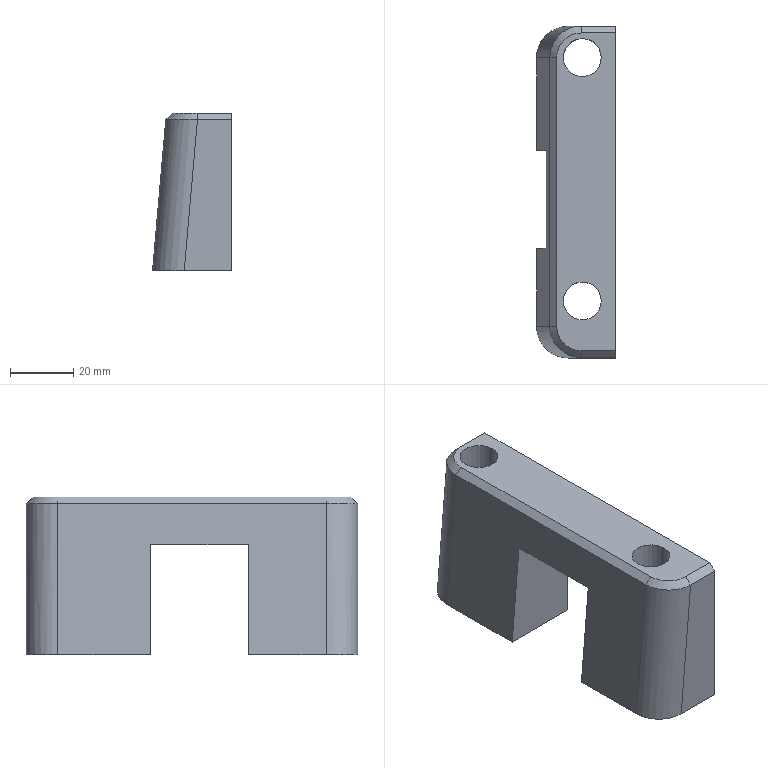Part | STEP file | solid 75 | 1 solid | 23 faces | box 25 x 105 x 50 mm | volume 77206 mm3 | plane 15 | cylinder 6 | spline 2 | commonest cylinder face diameters 12 x2 18 x2 20 x2